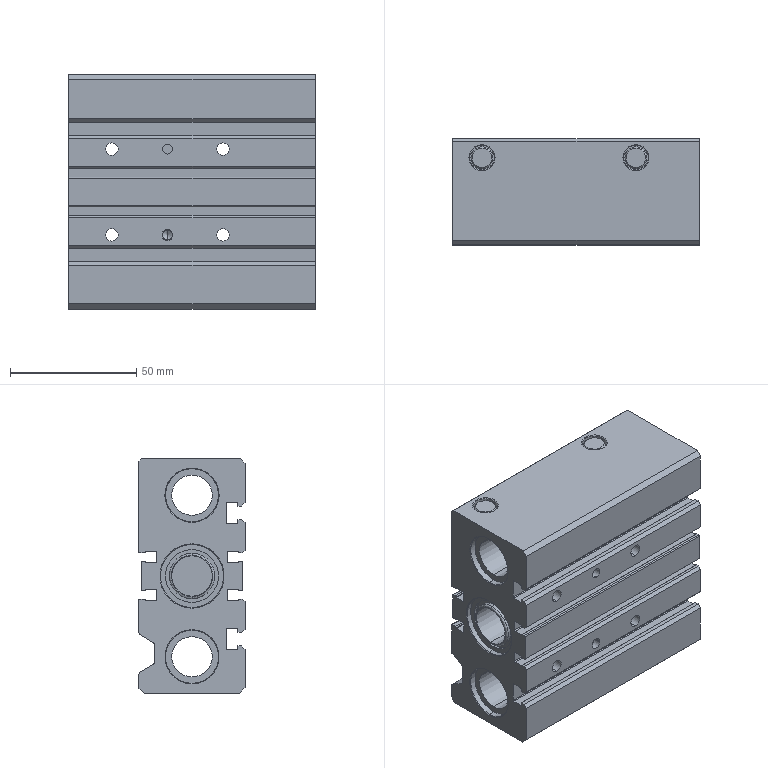Part | SolidWorks | features BaseBody 1 | 1 solid | 292 faces | box 97.5 x 42 x 93 mm | volume 253511 mm3 | cylinder 132 | plane 96 | cone 60 | spline 4 | commonest cylinder face diameters 0.8 x28 4.917 x16 4 x14 0.4 x12 5.5 x8 9.5 x8